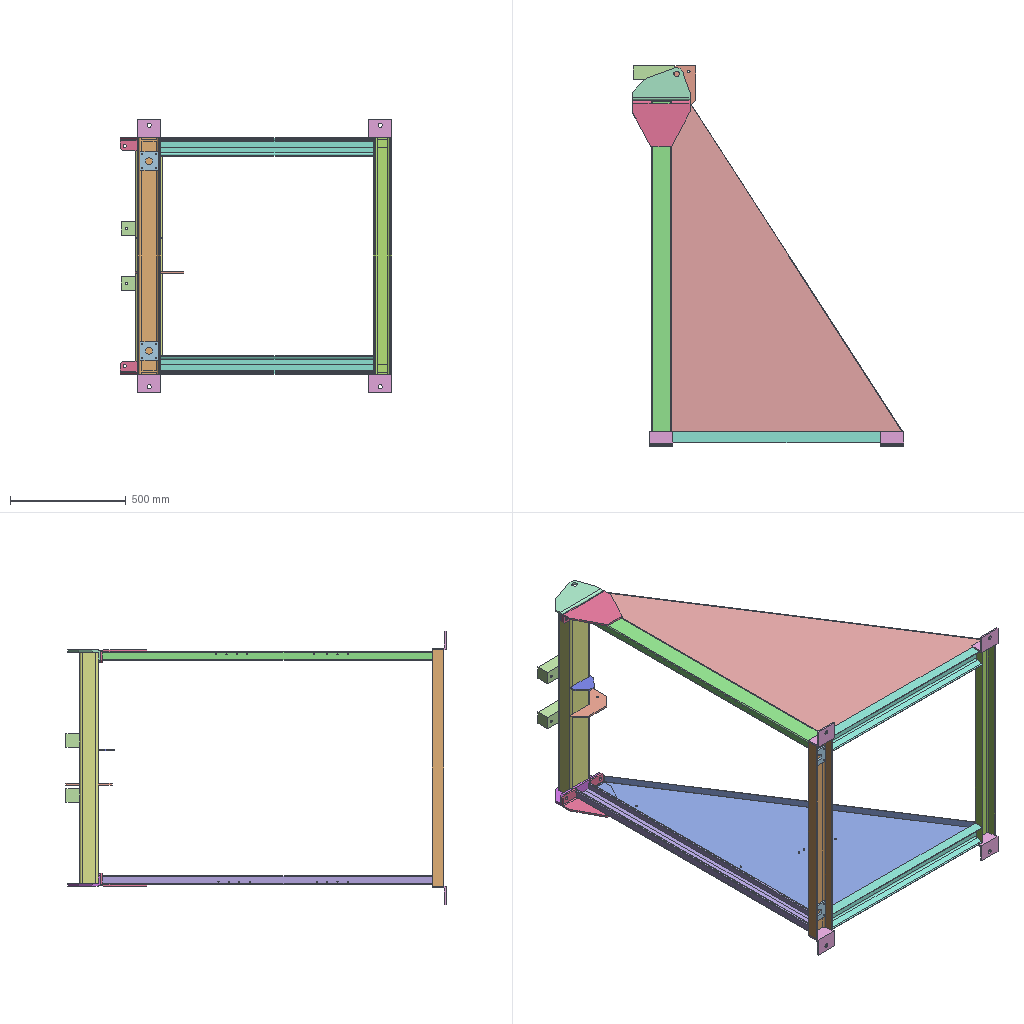Assembly | SolidWorks | 18 different items | 25 placed | box 1175 x 1645 x 1182 mm
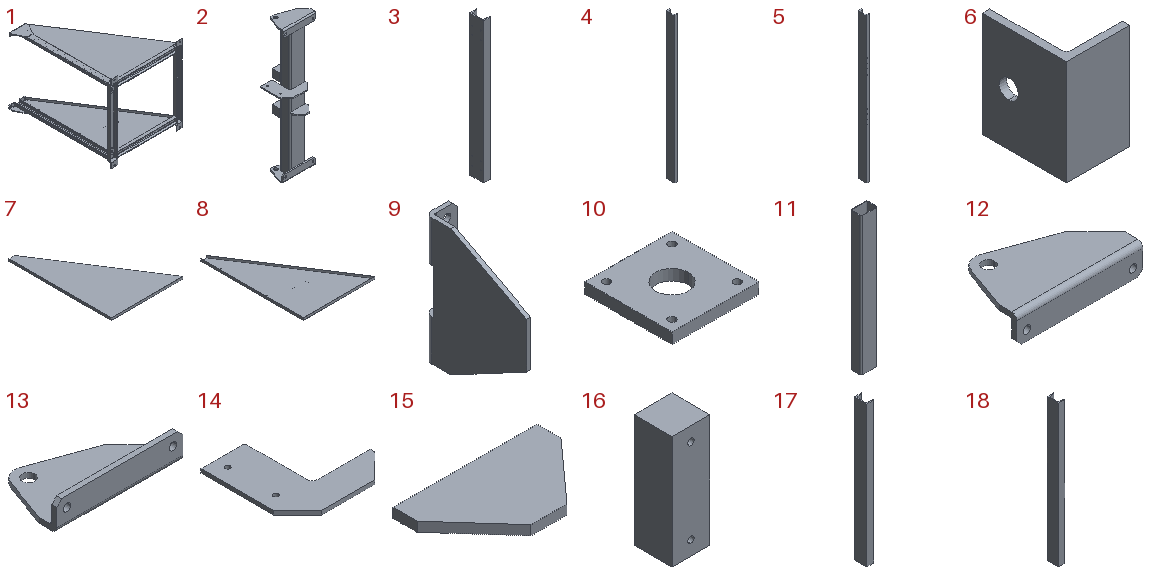Parts list (item | name | quantity | parent item | size | volume | features):
1 | (subassembly) | x1 | - | 1175 x 1495 x 1182 mm | 13027521 mm3 | -
2 | (subassembly) | x1 | - | 275 x 210 x 1022 mm | 3701713 mm3 | -
3 | - | x1 | in 1 | 50 x 100 x 1022 mm | 1354327 mm3 | features Extrusion 1, HoleWzd 1
4 | - | x1 | in 1 | 36 x 86.5 x 1430 mm | 1904339 mm3 | features Extrusion 1, HoleWzd 1
5 | - | x1 | in 1 | 36 x 86.5 x 1430 mm | 1904339 mm3 | features Extrusion 1, HoleWzd 1, ICE 1
6 | - | x4 | in 1 | 60 x 80 x 100 mm | 91855 mm3 | features Extrusion 1, Fillet 1, ICE 1
7 | - | x1 | in 1 | 1002 x 1427 x 32 mm | 1793698 mm3 | features ICE 2, Extrusion 1
8 | - | x1 | in 1 | 1002 x 1427 x 32 mm | 1793236 mm3 | features ICE 4, Extrusion 1
9 | - | x2 | in 1 | 55 x 200 x 250 mm | 345724 mm3 | features ICE 2, Chamfer 1, Extrusion 1
10 | - | x2 | in 1 | 80 x 80 x 10 mm | 55479 mm3 | features Extrusion 1, HoleWzd 1, ICE 1
11 | - | x1 | in 2 | 120 x 80 x 1002 mm | 1484024 mm3 | features Extrusion 1, Fillet 1, Shell 1
12 | - | x1 | in 2 | 250 x 141.5 x 55 mm | 355868 mm3 | features ICE 4, Fillet 2, Chamfer 1, Extrusion 1
13 | - | x1 | in 2 | 250 x 141.5 x 55 mm | 355868 mm3 | features ICE 4, Fillet 2, Chamfer 1, Extrusion 1
14 | - | x1 | in 2 | 210 x 200 x 8 mm | 180364 mm3 | features Chamfer 2, Extrusion 1, Fillet 1, HoleWzd 1, ICE 1
15 | - | x1 | in 2 | 120 x 70 x 8 mm | 49200 mm3 | features Extrusion 1, ICE 1
16 | - | x2 | in 2 | 60 x 60 x 180 mm | 638194 mm3 | features Extrusion 1, HoleWzd 1
17 | - | x2 | in 1 | 45 x 80 x 920 mm | 998999 mm3 | features Extrusion 1
18 | - | x1 | in 1 | 45 x 80 x 1022 mm | 1109758 mm3 | features Extrusion 1
Mates (type | each side: item.copy, entity, surface, feature):
In the top assembly
Coincident | 9.1 face plane Boss-Extrude1 | 13.1 face plane Boss-Extrude1
Concentric | 9.1 face cylinder Cut-Extrude2 | 13.1 face cylinder Cut-Extrude4
Concentric | 9.2 face cylinder Cut-Extrude2 | 12.1 face cylinder Cut-Extrude3
In subassembly 2
Coincident | 11.1 face plane Boss-Extrude1 | 12.2 face plane Boss-Extrude1
Coincident | 11.1 face plane Boss-Extrude1 | 13.2 face plane Boss-Extrude1
Coincident | 12.2 face plane Boss-Extrude1 | 13.2 face plane Boss-Extrude1
Coincident | 12.2 face plane Boss-Extrude2 | 13.2 face plane Boss-Extrude3
Coincident | 11.1 face plane Boss-Extrude1 | 12.2 face plane Boss-Extrude2
DistanceDim | 12.2 face plane Boss-Extrude1 | 11.1 face plane Boss-Extrude1
Coincident | 11.1 face plane Boss-Extrude1 | 14.1 face plane Cut-Extrude1 | 2 times
Coincident | 11.1 face plane Boss-Extrude1 | 15.1 face plane Boss-Extrude1 | 2 times
DistanceDim | 14.1 face plane Boss-Extrude1 | 13.2 face plane Boss-Extrude1
Coincident | 11.1 face plane Boss-Extrude1 | 16.1 face plane Boss-Extrude1 | 2 times
Coincident | 11.1 face plane Boss-Extrude1 | 16.2 face plane Boss-Extrude1
Coincident | 16.1 face plane Boss-Extrude1 | 16.2 face plane Boss-Extrude1
Parallel | 11.1 face plane Boss-Extrude1 | 16.2 face plane Boss-Extrude1
DistanceDim | 16.2 face plane Boss-Extrude1 | 16.1 face plane Boss-Extrude1
DistanceDim | 16.1 face plane Boss-Extrude1 | 12.2 face plane Boss-Extrude1
DistanceDim | 15.1 face plane Boss-Extrude1 | 16.1 face plane Boss-Extrude1
In subassembly 1
Coincident | 7.1 face plane Boss-Extrude1 | 8.1 face plane Boss-Extrude1 | 2 times
Coincident | 7.1 face plane Boss-Extrude1 | 18.1 face plane Boss-Extrude1
Coincident | 18.1 face plane Boss-Extrude1 | 6.1 face plane Boss-Extrude1 | 2 times
Parallel | 18.1 face plane Boss-Extrude1 | 6.1 face plane Boss-Extrude1
Coincident | 18.1 face plane Boss-Extrude1 | 17.1 face plane Boss-Extrude1 | 2 times
Coincident | 18.1 face plane Boss-Extrude1 | 17.2 face plane Boss-Extrude1 | 3 times
Coincident | 6.1 face plane Boss-Extrude1 | 17.1 face plane Boss-Extrude1
DistanceDim | 8.1 face plane Boss-Extrude1 | 17.2 face plane Boss-Extrude1
DistanceDim | 7.1 face plane Boss-Extrude1 | 17.1 face plane Boss-Extrude1
Coincident | 17.1 face plane Boss-Extrude1 | 3.1 face plane Boss-Extrude1 | 2 times
Coincident | 17.2 face plane Boss-Extrude1 | 3.1 face plane Boss-Extrude1
Coincident | 3.1 face plane Boss-Extrude1 | 4.1 face plane Boss-Extrude1
Coincident | 8.1 face plane Boss-Extrude1 | 4.1 face plane Boss-Extrude1 | 2 times
Coincident | 3.1 face plane Boss-Extrude1 | 5.1 face plane Boss-Extrude1
Coincident | 7.1 face plane Boss-Extrude1 | 5.1 face plane Boss-Extrude1 | 2 times
Coincident | 17.1 face plane Boss-Extrude1 | 6.2 face plane Boss-Extrude1
Coincident | 3.1 face plane Boss-Extrude1 | 6.2 face plane Boss-Extrude1
Coincident | 6.1 face plane Boss-Extrude1 | 6.2 face plane Boss-Extrude1
Coincident | 6.3 face plane Boss-Extrude1 | 6.4 face plane Boss-Extrude1 | 2 times
Coincident | 17.2 face plane Boss-Extrude1 | 6.4 face plane Boss-Extrude1
Coincident | 3.1 face plane Boss-Extrude1 | 6.4 face plane Boss-Extrude1
Coincident | 18.1 face plane Boss-Extrude1 | 6.3 face plane Boss-Extrude1 | 2 times
Coincident | 6.1 face plane Boss-Extrude1 | 6.3 face plane Boss-Extrude1
Coincident | 5.1 face plane Boss-Extrude1 | 9.3 face plane Boss-Extrude1
Coincident | 5.1 face plane Boss-Extrude1 | 9.3 face plane Cut-Extrude1
Coincident | 7.1 edge | 9.3 face plane Boss-Extrude1
Coincident | 9.3 face plane Boss-Extrude1 | 9.4 face plane Boss-Extrude1 | 2 times
Coincident | 4.1 face plane Boss-Extrude1 | 9.4 face plane Boss-Extrude1
Coincident | 3.1 face plane Boss-Extrude1 | 10.1 face plane Boss-Extrude1
Coincident | 10.1 face plane Boss-Extrude1 | 10.2 face plane Boss-Extrude1 | 2 times
Concentric | 3.1 face cylinder M8 Tapped Hole1 | 10.1 face cylinder M8 Tapped Hole1 | 2 times
Concentric | 3.1 face cylinder M8 Tapped Hole1 | 10.2 face cylinder M8 Tapped Hole1 | 2 times
Width | 3.1 face plane Boss-Extrude1 | 3.1 face plane Boss-Extrude1 | 5.1 face plane Boss-Extrude1 | 5.1 face plane Boss-Extrude1